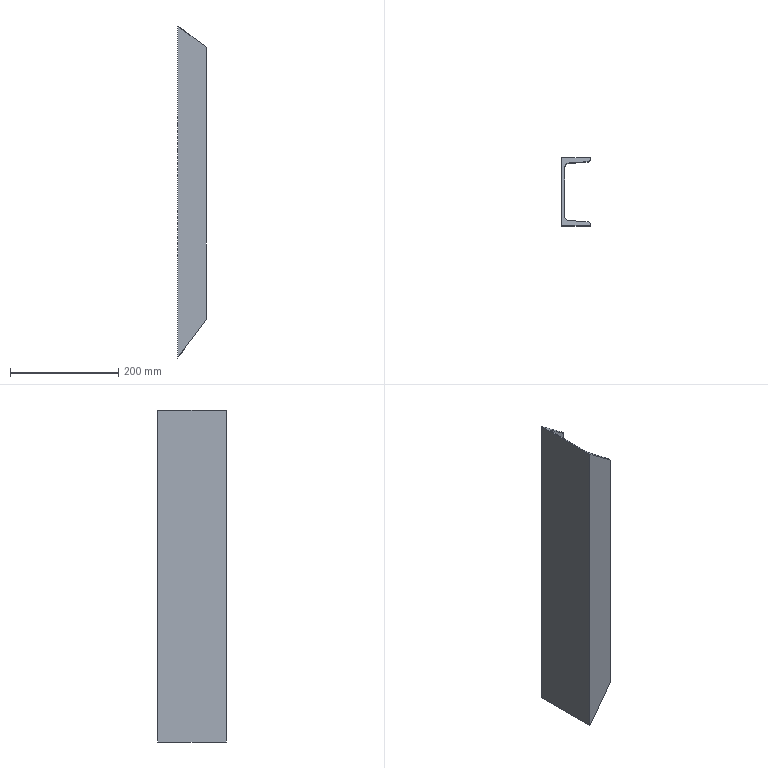Part | SolidWorks | features Extrusion 1, ICE 1 | 1 solid | 14 faces | box 53 x 126 x 613 mm | volume 899229 mm3 | plane 10 | cylinder 4 | commonest cylinder face diameters 9 x2 18 x2
STEP:
#1=CARTESIAN_POINT('',(53.,63.,267.21));
#2=VERTEX_POINT('',#1);
#3=CARTESIAN_POINT('',(53.,63.,-235.005));
#4=VERTEX_POINT('',#3);
#5=CARTESIAN_POINT('',(53.,63.,306.5));
#6=DIRECTION('',(0.,0.,-1.));
#7=VECTOR('',#6,1000.);
#8=LINE('',#5,#7);
#9=EDGE_CURVE('',#2,#4,#8,.T.);
#10=ORIENTED_EDGE('',*,*,#9,.T.);
#11=CARTESIAN_POINT('',(0.,63.,-306.5));
#12=VERTEX_POINT('',#11);
#13=CARTESIAN_POINT('',(0.,63.,-306.5));
#14=DIRECTION('',(0.5955,0.,0.8033));
#15=VECTOR('',#14,1000.);
#16=LINE('',#13,#15);
#17=EDGE_CURVE('',#12,#4,#16,.T.);
#18=ORIENTED_EDGE('',*,*,#17,.F.);
#19=CARTESIAN_POINT('',(0.,63.,306.5));
#20=VERTEX_POINT('',#19);
#21=CARTESIAN_POINT('',(0.,63.,306.5));
#22=DIRECTION('',(0.,0.,-1.));
#23=VECTOR('',#22,1000.);
#24=LINE('',#21,#23);
#25=EDGE_CURVE('',#20,#12,#24,.T.);
#26=ORIENTED_EDGE('',*,*,#25,.F.);
#27=CARTESIAN_POINT('',(0.,63.,306.5));
#28=DIRECTION('',(-0.8033,0.,0.5955));
#29=VECTOR('',#28,1000.);
#30=LINE('',#27,#29);
#31=EDGE_CURVE('',#2,#20,#30,.T.);
#32=ORIENTED_EDGE('',*,*,#31,.F.);
#33=EDGE_LOOP('',(#10,#18,#26,#32));
#34=FACE_OUTER_BOUND('',#33,.T.);
#35=CARTESIAN_POINT('',(0.,63.,306.5));
#36=DIRECTION('',(0.,-1.,0.));
#37=DIRECTION('',(0.,0.,-1.));
#38=AXIS2_PLACEMENT_3D('',#35,#36,#37);
#39=PLANE('',#38);
#40=ADVANCED_FACE('',(#34),#39,.F.);
#41=CARTESIAN_POINT('',(0.,-63.,-306.5));
#42=VERTEX_POINT('',#41);
#43=CARTESIAN_POINT('',(0.,63.,-306.5));
#44=DIRECTION('',(0.,-1.,0.));
#45=VECTOR('',#44,1000.);
#46=LINE('',#43,#45);
#47=EDGE_CURVE('',#12,#42,#46,.T.);
#48=ORIENTED_EDGE('',*,*,#47,.T.);
#49=CARTESIAN_POINT('',(0.,-63.,306.5));
#50=VERTEX_POINT('',#49);
#51=CARTESIAN_POINT('',(0.,-63.,306.5));
#52=DIRECTION('',(0.,0.,-1.));
#53=VECTOR('',#52,1000.);
#54=LINE('',#51,#53);
#55=EDGE_CURVE('',#50,#42,#54,.T.);
#56=ORIENTED_EDGE('',*,*,#55,.F.);
#57=CARTESIAN_POINT('',(0.,63.,306.5));
#58=DIRECTION('',(0.,-1.,0.));
#59=VECTOR('',#58,1000.);
#60=LINE('',#57,#59);
#61=EDGE_CURVE('',#20,#50,#60,.T.);
#62=ORIENTED_EDGE('',*,*,#61,.F.);
#63=ORIENTED_EDGE('',*,*,#25,.T.);
#64=EDGE_LOOP('',(#48,#56,#62,#63));
#65=FACE_OUTER_BOUND('',#64,.T.);
#66=CARTESIAN_POINT('',(0.,63.,306.5));
#67=DIRECTION('',(1.,0.,0.));
#68=DIRECTION('',(0.,0.,-1.));
#69=AXIS2_PLACEMENT_3D('',#66,#67,#68);
#70=PLANE('',#69);
#71=ADVANCED_FACE('',(#65),#70,.F.);
#72=ORIENTED_EDGE('',*,*,#55,.T.);
#73=CARTESIAN_POINT('',(53.,-63.,-235.005));
#74=VERTEX_POINT('',#73);
#75=CARTESIAN_POINT('',(293.263,-63.,89.1));
#76=DIRECTION('',(0.5955,0.,0.8033));
#77=VECTOR('',#76,1000.);
#78=LINE('',#75,#77);
#79=EDGE_CURVE('',#42,#74,#78,.T.);
#80=ORIENTED_EDGE('',*,*,#79,.T.);
#81=CARTESIAN_POINT('',(53.,-63.,267.21));
#82=VERTEX_POINT('',#81);
#83=CARTESIAN_POINT('',(53.,-63.,306.5));
#84=DIRECTION('',(0.,0.,-1.));
#85=VECTOR('',#84,1000.);
#86=LINE('',#83,#85);
#87=EDGE_CURVE('',#82,#74,#86,.T.);
#88=ORIENTED_EDGE('',*,*,#87,.F.);
#89=CARTESIAN_POINT('',(0.,-63.,306.5));
#90=DIRECTION('',(-0.8033,0.,0.5955));
#91=VECTOR('',#90,1000.);
#92=LINE('',#89,#91);
#93=EDGE_CURVE('',#82,#50,#92,.T.);
#94=ORIENTED_EDGE('',*,*,#93,.T.);
#95=EDGE_LOOP('',(#72,#80,#88,#94));
#96=FACE_OUTER_BOUND('',#95,.T.);
#97=CARTESIAN_POINT('',(0.,-63.,306.5));
#98=DIRECTION('',(0.,1.,0.));
#99=DIRECTION('',(0.,0.,1.));
#100=AXIS2_PLACEMENT_3D('',#97,#98,#99);
#101=PLANE('',#100);
#102=ADVANCED_FACE('',(#96),#101,.F.);
#103=ORIENTED_EDGE('',*,*,#87,.T.);
#104=CARTESIAN_POINT('',(53.,-60.016,-235.005));
#105=VERTEX_POINT('',#104);
#106=CARTESIAN_POINT('',(53.,-550.,-235.005));
#107=DIRECTION('',(0.,1.,0.));
#108=VECTOR('',#107,1000.);
#109=LINE('',#106,#108);
#110=EDGE_CURVE('',#74,#105,#109,.T.);
#111=ORIENTED_EDGE('',*,*,#110,.T.);
#112=CARTESIAN_POINT('',(53.,-60.016,267.21));
#113=VERTEX_POINT('',#112);
#114=CARTESIAN_POINT('',(53.,-60.016,306.5));
#115=DIRECTION('',(0.,0.,-1.));
#116=VECTOR('',#115,1000.);
#117=LINE('',#114,#116);
#118=EDGE_CURVE('',#113,#105,#117,.T.);
#119=ORIENTED_EDGE('',*,*,#118,.F.);
#120=CARTESIAN_POINT('',(53.,-550.,267.21));
#121=DIRECTION('',(0.,1.,0.));
#122=VECTOR('',#121,1000.);
#123=LINE('',#120,#122);
#124=EDGE_CURVE('',#82,#113,#123,.T.);
#125=ORIENTED_EDGE('',*,*,#124,.F.);
#126=EDGE_LOOP('',(#103,#111,#119,#125));
#127=FACE_OUTER_BOUND('',#126,.T.);
#128=CARTESIAN_POINT('',(53.,-63.,306.5));
#129=DIRECTION('',(-1.,0.,0.));
#130=DIRECTION('',(0.,0.,1.));
#131=AXIS2_PLACEMENT_3D('',#128,#129,#130);
#132=PLANE('',#131);
#133=ADVANCED_FACE('',(#127),#132,.F.);
#134=ORIENTED_EDGE('',*,*,#118,.T.);
#135=CARTESIAN_POINT('',(48.807,-55.526,-240.662));
#136=VERTEX_POINT('',#135);
#137=CARTESIAN_POINT('',(53.,-60.016,-235.005));
#138=CARTESIAN_POINT('',(53.,-57.52,-235.005));
#139=CARTESIAN_POINT('',(51.297,-55.697,-237.303));
#140=CARTESIAN_POINT('',(48.807,-55.526,-240.662));
#141=(BOUNDED_CURVE()B_SPLINE_CURVE(3,(#137,#138,#139,#140),.UNSPECIFIED.,.F.,.T.)B_SPLINE_CURVE_WITH_KNOTS((4,4),(3.142,4.644),.UNSPECIFIED.)CURVE()GEOMETRIC_REPRESENTATION_ITEM()RATIONAL_B_SPLINE_CURVE((1.,0.8205,0.8205,1.))REPRESENTATION_ITEM(''));
#142=EDGE_CURVE('',#105,#136,#141,.T.);
#143=ORIENTED_EDGE('',*,*,#142,.T.);
#144=CARTESIAN_POINT('',(48.807,-55.526,270.319));
#145=VERTEX_POINT('',#144);
#146=CARTESIAN_POINT('',(48.807,-55.526,306.5));
#147=DIRECTION('',(0.,0.,-1.));
#148=VECTOR('',#147,1000.);
#149=LINE('',#146,#148);
#150=EDGE_CURVE('',#145,#136,#149,.T.);
#151=ORIENTED_EDGE('',*,*,#150,.F.);
#152=CARTESIAN_POINT('',(48.807,-55.526,270.319));
#153=CARTESIAN_POINT('',(51.297,-55.697,268.473));
#154=CARTESIAN_POINT('',(53.,-57.52,267.21));
#155=CARTESIAN_POINT('',(53.,-60.016,267.21));
#156=(BOUNDED_CURVE()B_SPLINE_CURVE(3,(#152,#153,#154,#155),.UNSPECIFIED.,.F.,.T.)B_SPLINE_CURVE_WITH_KNOTS((4,4),(4.781,6.283),.UNSPECIFIED.)CURVE()GEOMETRIC_REPRESENTATION_ITEM()RATIONAL_B_SPLINE_CURVE((1.,0.8205,0.8205,1.))REPRESENTATION_ITEM(''));
#157=EDGE_CURVE('',#145,#113,#156,.T.);
#158=ORIENTED_EDGE('',*,*,#157,.T.);
#159=EDGE_LOOP('',(#134,#143,#151,#158));
#160=FACE_OUTER_BOUND('',#159,.T.);
#161=CARTESIAN_POINT('',(48.5,-60.016,306.5));
#162=DIRECTION('',(0.,0.,-1.));
#163=DIRECTION('',(-1.,0.,0.));
#164=AXIS2_PLACEMENT_3D('',#161,#162,#163);
#165=CYLINDRICAL_SURFACE('',#164,4.5);
#166=ADVANCED_FACE('',(#160),#165,.T.);
#167=ORIENTED_EDGE('',*,*,#150,.T.);
#168=CARTESIAN_POINT('',(13.886,-53.14,-287.768));
#169=VERTEX_POINT('',#168);
#170=CARTESIAN_POINT('',(310.14,-73.388,111.866));
#171=DIRECTION('',(-0.595,0.04067,-0.8027));
#172=VECTOR('',#171,1000.);
#173=LINE('',#170,#172);
#174=EDGE_CURVE('',#136,#169,#173,.T.);
#175=ORIENTED_EDGE('',*,*,#174,.T.);
#176=CARTESIAN_POINT('',(13.886,-53.14,296.206));
#177=VERTEX_POINT('',#176);
#178=CARTESIAN_POINT('',(13.886,-53.14,306.5));
#179=DIRECTION('',(0.,0.,-1.));
#180=VECTOR('',#179,1000.);
#181=LINE('',#178,#180);
#182=EDGE_CURVE('',#177,#169,#181,.T.);
#183=ORIENTED_EDGE('',*,*,#182,.F.);
#184=CARTESIAN_POINT('',(31.55,-54.347,283.112));
#185=DIRECTION('',(0.8021,-0.05482,-0.5946));
#186=VECTOR('',#185,1000.);
#187=LINE('',#184,#186);
#188=EDGE_CURVE('',#177,#145,#187,.T.);
#189=ORIENTED_EDGE('',*,*,#188,.T.);
#190=EDGE_LOOP('',(#167,#175,#183,#189));
#191=FACE_OUTER_BOUND('',#190,.T.);
#192=CARTESIAN_POINT('',(48.807,-55.526,306.5));
#193=DIRECTION('',(-0.06819,-0.9977,0.));
#194=DIRECTION('',(0.9977,-0.06819,0.));
#195=AXIS2_PLACEMENT_3D('',#192,#193,#194);
#196=PLANE('',#195);
#197=ADVANCED_FACE('',(#191),#196,.F.);
#198=ORIENTED_EDGE('',*,*,#182,.T.);
#199=CARTESIAN_POINT('',(5.5,-44.161,-299.081));
#200=VERTEX_POINT('',#199);
#201=CARTESIAN_POINT('',(13.886,-53.14,-287.768));
#202=CARTESIAN_POINT('',(8.907,-52.799,-294.485));
#203=CARTESIAN_POINT('',(5.5,-49.152,-299.081));
#204=CARTESIAN_POINT('',(5.5,-44.161,-299.081));
#205=(BOUNDED_CURVE()B_SPLINE_CURVE(3,(#201,#202,#203,#204),.UNSPECIFIED.,.F.,.F.)B_SPLINE_CURVE_WITH_KNOTS((4,4),(4.781,6.283),.UNSPECIFIED.)CURVE()GEOMETRIC_REPRESENTATION_ITEM()RATIONAL_B_SPLINE_CURVE((1.,0.8205,0.8205,1.))REPRESENTATION_ITEM(''));
#206=EDGE_CURVE('',#169,#200,#205,.T.);
#207=ORIENTED_EDGE('',*,*,#206,.T.);
#208=CARTESIAN_POINT('',(5.5,-44.161,302.423));
#209=VERTEX_POINT('',#208);
#210=CARTESIAN_POINT('',(5.5,-44.161,306.5));
#211=DIRECTION('',(0.,0.,-1.));
#212=VECTOR('',#211,1000.);
#213=LINE('',#210,#212);
#214=EDGE_CURVE('',#209,#200,#213,.T.);
#215=ORIENTED_EDGE('',*,*,#214,.F.);
#216=CARTESIAN_POINT('',(5.5,-44.161,302.423));
#217=CARTESIAN_POINT('',(5.5,-49.152,302.423));
#218=CARTESIAN_POINT('',(8.907,-52.799,299.897));
#219=CARTESIAN_POINT('',(13.886,-53.14,296.206));
#220=(BOUNDED_CURVE()B_SPLINE_CURVE(3,(#216,#217,#218,#219),.UNSPECIFIED.,.F.,.T.)B_SPLINE_CURVE_WITH_KNOTS((4,4),(3.142,4.644),.UNSPECIFIED.)CURVE()GEOMETRIC_REPRESENTATION_ITEM()RATIONAL_B_SPLINE_CURVE((1.,0.8205,0.8205,1.))REPRESENTATION_ITEM(''));
#221=EDGE_CURVE('',#209,#177,#220,.T.);
#222=ORIENTED_EDGE('',*,*,#221,.T.);
#223=EDGE_LOOP('',(#198,#207,#215,#222));
#224=FACE_OUTER_BOUND('',#223,.T.);
#225=CARTESIAN_POINT('',(14.5,-44.161,306.5));
#226=DIRECTION('',(0.,0.,-1.));
#227=DIRECTION('',(-1.,0.,0.));
#228=AXIS2_PLACEMENT_3D('',#225,#226,#227);
#229=CYLINDRICAL_SURFACE('',#228,9.);
#230=ADVANCED_FACE('',(#224),#229,.F.);
#231=ORIENTED_EDGE('',*,*,#214,.T.);
#232=CARTESIAN_POINT('',(5.5,44.161,-299.081));
#233=VERTEX_POINT('',#232);
#234=CARTESIAN_POINT('',(5.5,44.161,-299.081));
#235=DIRECTION('',(0.,1.,0.));
#236=VECTOR('',#235,1000.);
#237=LINE('',#234,#236);
#238=EDGE_CURVE('',#200,#233,#237,.T.);
#239=ORIENTED_EDGE('',*,*,#238,.T.);
#240=CARTESIAN_POINT('',(5.5,44.161,302.423));
#241=VERTEX_POINT('',#240);
#242=CARTESIAN_POINT('',(5.5,44.161,306.5));
#243=DIRECTION('',(0.,0.,-1.));
#244=VECTOR('',#243,1000.);
#245=LINE('',#242,#244);
#246=EDGE_CURVE('',#241,#233,#245,.T.);
#247=ORIENTED_EDGE('',*,*,#246,.F.);
#248=CARTESIAN_POINT('',(5.5,44.161,302.423));
#249=DIRECTION('',(0.,-1.,0.));
#250=VECTOR('',#249,1000.);
#251=LINE('',#248,#250);
#252=EDGE_CURVE('',#241,#209,#251,.T.);
#253=ORIENTED_EDGE('',*,*,#252,.T.);
#254=EDGE_LOOP('',(#231,#239,#247,#253));
#255=FACE_OUTER_BOUND('',#254,.T.);
#256=CARTESIAN_POINT('',(5.5,44.161,306.5));
#257=DIRECTION('',(-1.,0.,0.));
#258=DIRECTION('',(0.,-1.,0.));
#259=AXIS2_PLACEMENT_3D('',#256,#257,#258);
#260=PLANE('',#259);
#261=ADVANCED_FACE('',(#255),#260,.F.);
#262=ORIENTED_EDGE('',*,*,#246,.T.);
#263=CARTESIAN_POINT('',(13.886,53.14,-287.768));
#264=VERTEX_POINT('',#263);
#265=CARTESIAN_POINT('',(5.5,44.161,-299.081));
#266=CARTESIAN_POINT('',(5.5,49.152,-299.081));
#267=CARTESIAN_POINT('',(8.907,52.799,-294.485));
#268=CARTESIAN_POINT('',(13.886,53.14,-287.768));
#269=(BOUNDED_CURVE()B_SPLINE_CURVE(3,(#265,#266,#267,#268),.UNSPECIFIED.,.F.,.F.)B_SPLINE_CURVE_WITH_KNOTS((4,4),(0.,1.503),.UNSPECIFIED.)CURVE()GEOMETRIC_REPRESENTATION_ITEM()RATIONAL_B_SPLINE_CURVE((1.,0.8205,0.8205,1.))REPRESENTATION_ITEM(''));
#270=EDGE_CURVE('',#233,#264,#269,.T.);
#271=ORIENTED_EDGE('',*,*,#270,.T.);
#272=CARTESIAN_POINT('',(13.886,53.14,296.206));
#273=VERTEX_POINT('',#272);
#274=CARTESIAN_POINT('',(13.886,53.14,306.5));
#275=DIRECTION('',(0.,0.,-1.));
#276=VECTOR('',#275,1000.);
#277=LINE('',#274,#276);
#278=EDGE_CURVE('',#273,#264,#277,.T.);
#279=ORIENTED_EDGE('',*,*,#278,.F.);
#280=CARTESIAN_POINT('',(13.886,53.14,296.206));
#281=CARTESIAN_POINT('',(8.907,52.799,299.897));
#282=CARTESIAN_POINT('',(5.5,49.152,302.423));
#283=CARTESIAN_POINT('',(5.5,44.161,302.423));
#284=(BOUNDED_CURVE()B_SPLINE_CURVE(3,(#280,#281,#282,#283),.UNSPECIFIED.,.F.,.T.)B_SPLINE_CURVE_WITH_KNOTS((4,4),(1.639,3.142),.UNSPECIFIED.)CURVE()GEOMETRIC_REPRESENTATION_ITEM()RATIONAL_B_SPLINE_CURVE((1.,0.8205,0.8205,1.))REPRESENTATION_ITEM(''));
#285=EDGE_CURVE('',#273,#241,#284,.T.);
#286=ORIENTED_EDGE('',*,*,#285,.T.);
#287=EDGE_LOOP('',(#262,#271,#279,#286));
#288=FACE_OUTER_BOUND('',#287,.T.);
#289=CARTESIAN_POINT('',(14.5,44.161,306.5));
#290=DIRECTION('',(0.,0.,-1.));
#291=DIRECTION('',(-1.,0.,0.));
#292=AXIS2_PLACEMENT_3D('',#289,#290,#291);
#293=CYLINDRICAL_SURFACE('',#292,9.);
#294=ADVANCED_FACE('',(#288),#293,.F.);
#295=ORIENTED_EDGE('',*,*,#278,.T.);
#296=CARTESIAN_POINT('',(48.807,55.526,-240.662));
#297=VERTEX_POINT('',#296);
#298=CARTESIAN_POINT('',(310.14,73.388,111.866));
#299=DIRECTION('',(0.595,0.04067,0.8027));
#300=VECTOR('',#299,1000.);
#301=LINE('',#298,#300);
#302=EDGE_CURVE('',#264,#297,#301,.T.);
#303=ORIENTED_EDGE('',*,*,#302,.T.);
#304=CARTESIAN_POINT('',(48.807,55.526,270.319));
#305=VERTEX_POINT('',#304);
#306=CARTESIAN_POINT('',(48.807,55.526,306.5));
#307=DIRECTION('',(0.,0.,-1.));
#308=VECTOR('',#307,1000.);
#309=LINE('',#306,#308);
#310=EDGE_CURVE('',#305,#297,#309,.T.);
#311=ORIENTED_EDGE('',*,*,#310,.F.);
#312=CARTESIAN_POINT('',(31.55,54.347,283.112));
#313=DIRECTION('',(-0.8021,-0.05482,0.5946));
#314=VECTOR('',#313,1000.);
#315=LINE('',#312,#314);
#316=EDGE_CURVE('',#305,#273,#315,.T.);
#317=ORIENTED_EDGE('',*,*,#316,.T.);
#318=EDGE_LOOP('',(#295,#303,#311,#317));
#319=FACE_OUTER_BOUND('',#318,.T.);
#320=CARTESIAN_POINT('',(48.807,55.526,306.5));
#321=DIRECTION('',(-0.06819,0.9977,0.));
#322=DIRECTION('',(-0.9977,-0.06819,0.));
#323=AXIS2_PLACEMENT_3D('',#320,#321,#322);
#324=PLANE('',#323);
#325=ADVANCED_FACE('',(#319),#324,.F.);
#326=ORIENTED_EDGE('',*,*,#310,.T.);
#327=CARTESIAN_POINT('',(53.,60.016,-235.005));
#328=VERTEX_POINT('',#327);
#329=CARTESIAN_POINT('',(48.807,55.526,-240.662));
#330=CARTESIAN_POINT('',(51.297,55.697,-237.303));
#331=CARTESIAN_POINT('',(53.,57.52,-235.005));
#332=CARTESIAN_POINT('',(53.,60.016,-235.005));
#333=(BOUNDED_CURVE()B_SPLINE_CURVE(3,(#329,#330,#331,#332),.UNSPECIFIED.,.F.,.T.)B_SPLINE_CURVE_WITH_KNOTS((4,4),(1.639,3.142),.UNSPECIFIED.)CURVE()GEOMETRIC_REPRESENTATION_ITEM()RATIONAL_B_SPLINE_CURVE((1.,0.8205,0.8205,1.))REPRESENTATION_ITEM(''));
#334=EDGE_CURVE('',#297,#328,#333,.T.);
#335=ORIENTED_EDGE('',*,*,#334,.T.);
#336=CARTESIAN_POINT('',(53.,60.016,267.21));
#337=VERTEX_POINT('',#336);
#338=CARTESIAN_POINT('',(53.,60.016,306.5));
#339=DIRECTION('',(0.,0.,-1.));
#340=VECTOR('',#339,1000.);
#341=LINE('',#338,#340);
#342=EDGE_CURVE('',#337,#328,#341,.T.);
#343=ORIENTED_EDGE('',*,*,#342,.F.);
#344=CARTESIAN_POINT('',(53.,60.016,267.21));
#345=CARTESIAN_POINT('',(53.,57.52,267.21));
#346=CARTESIAN_POINT('',(51.297,55.697,268.473));
#347=CARTESIAN_POINT('',(48.807,55.526,270.319));
#348=(BOUNDED_CURVE()B_SPLINE_CURVE(3,(#344,#345,#346,#347),.UNSPECIFIED.,.F.,.T.)B_SPLINE_CURVE_WITH_KNOTS((4,4),(0.,1.503),.UNSPECIFIED.)CURVE()GEOMETRIC_REPRESENTATION_ITEM()RATIONAL_B_SPLINE_CURVE((1.,0.8205,0.8205,1.))REPRESENTATION_ITEM(''));
#349=EDGE_CURVE('',#337,#305,#348,.T.);
#350=ORIENTED_EDGE('',*,*,#349,.T.);
#351=EDGE_LOOP('',(#326,#335,#343,#350));
#352=FACE_OUTER_BOUND('',#351,.T.);
#353=CARTESIAN_POINT('',(48.5,60.016,306.5));
#354=DIRECTION('',(0.,0.,-1.));
#355=DIRECTION('',(-1.,0.,0.));
#356=AXIS2_PLACEMENT_3D('',#353,#354,#355);
#357=CYLINDRICAL_SURFACE('',#356,4.5);
#358=ADVANCED_FACE('',(#352),#357,.T.);
#359=ORIENTED_EDGE('',*,*,#342,.T.);
#360=CARTESIAN_POINT('',(53.,-550.,-235.005));
#361=DIRECTION('',(0.,1.,0.));
#362=VECTOR('',#361,1000.);
#363=LINE('',#360,#362);
#364=EDGE_CURVE('',#328,#4,#363,.T.);
#365=ORIENTED_EDGE('',*,*,#364,.T.);
#366=ORIENTED_EDGE('',*,*,#9,.F.);
#367=CARTESIAN_POINT('',(53.,-550.,267.21));
#368=DIRECTION('',(0.,1.,0.));
#369=VECTOR('',#368,1000.);
#370=LINE('',#367,#369);
#371=EDGE_CURVE('',#337,#2,#370,.T.);
#372=ORIENTED_EDGE('',*,*,#371,.F.);
#373=EDGE_LOOP('',(#359,#365,#366,#372));
#374=FACE_OUTER_BOUND('',#373,.T.);
#375=CARTESIAN_POINT('',(53.,63.,306.5));
#376=DIRECTION('',(-1.,0.,0.));
#377=DIRECTION('',(0.,0.,1.));
#378=AXIS2_PLACEMENT_3D('',#375,#376,#377);
#379=PLANE('',#378);
#380=ADVANCED_FACE('',(#374),#379,.F.);
#381=ORIENTED_EDGE('',*,*,#124,.T.);
#382=ORIENTED_EDGE('',*,*,#157,.F.);
#383=ORIENTED_EDGE('',*,*,#188,.F.);
#384=ORIENTED_EDGE('',*,*,#221,.F.);
#385=ORIENTED_EDGE('',*,*,#252,.F.);
#386=ORIENTED_EDGE('',*,*,#285,.F.);
#387=ORIENTED_EDGE('',*,*,#316,.F.);
#388=ORIENTED_EDGE('',*,*,#349,.F.);
#389=ORIENTED_EDGE('',*,*,#371,.T.);
#390=ORIENTED_EDGE('',*,*,#31,.T.);
#391=ORIENTED_EDGE('',*,*,#61,.T.);
#392=ORIENTED_EDGE('',*,*,#93,.F.);
#393=EDGE_LOOP('',(#381,#382,#383,#384,#385,#386,#387,#388,#389,#390,#391,#392));
#394=FACE_OUTER_BOUND('',#393,.T.);
#395=CARTESIAN_POINT('',(0.,-550.,306.5));
#396=DIRECTION('',(-0.5955,0.,-0.8033));
#397=DIRECTION('',(-0.8033,0.,0.5955));
#398=AXIS2_PLACEMENT_3D('',#395,#396,#397);
#399=PLANE('',#398);
#400=ADVANCED_FACE('',(#394),#399,.F.);
#401=ORIENTED_EDGE('',*,*,#47,.F.);
#402=ORIENTED_EDGE('',*,*,#17,.T.);
#403=ORIENTED_EDGE('',*,*,#364,.F.);
#404=ORIENTED_EDGE('',*,*,#334,.F.);
#405=ORIENTED_EDGE('',*,*,#302,.F.);
#406=ORIENTED_EDGE('',*,*,#270,.F.);
#407=ORIENTED_EDGE('',*,*,#238,.F.);
#408=ORIENTED_EDGE('',*,*,#206,.F.);
#409=ORIENTED_EDGE('',*,*,#174,.F.);
#410=ORIENTED_EDGE('',*,*,#142,.F.);
#411=ORIENTED_EDGE('',*,*,#110,.F.);
#412=ORIENTED_EDGE('',*,*,#79,.F.);
#413=EDGE_LOOP('',(#401,#402,#403,#404,#405,#406,#407,#408,#409,#410,#411,#412));
#414=FACE_OUTER_BOUND('',#413,.T.);
#415=CARTESIAN_POINT('',(0.,-550.,-306.5));
#416=DIRECTION('',(-0.8033,0.,0.5955));
#417=DIRECTION('',(0.5955,0.,0.8033));
#418=AXIS2_PLACEMENT_3D('',#415,#416,#417);
#419=PLANE('',#418);
#420=ADVANCED_FACE('',(#414),#419,.F.);
#421=CLOSED_SHELL('',(#40,#71,#102,#133,#166,#197,#230,#261,#294,#325,#358,#380,#400,#420));
#422=MANIFOLD_SOLID_BREP('',#421);
#423=CARTESIAN_POINT('',(0.,0.,0.));
#424=DIRECTION('',(0.,0.,1.));
#425=DIRECTION('',(1.,0.,0.));
#426=AXIS2_PLACEMENT_3D('',#423,#424,#425);
#427=(LENGTH_UNIT()NAMED_UNIT(*)SI_UNIT(.MILLI.,.METRE.));
#428=UNCERTAINTY_MEASURE_WITH_UNIT(LENGTH_MEASURE(0.00001),#427,'','');
#429=(NAMED_UNIT(*)PLANE_ANGLE_UNIT()SI_UNIT($,.RADIAN.));
#430=(NAMED_UNIT(*)SI_UNIT($,.STERADIAN.)SOLID_ANGLE_UNIT());
#431=(GEOMETRIC_REPRESENTATION_CONTEXT(3)GLOBAL_UNCERTAINTY_ASSIGNED_CONTEXT((#428))GLOBAL_UNIT_ASSIGNED_CONTEXT((#427,#429,#430))REPRESENTATION_CONTEXT('',''));
#432=ADVANCED_BREP_SHAPE_REPRESENTATION('',(#422,#426),#431);